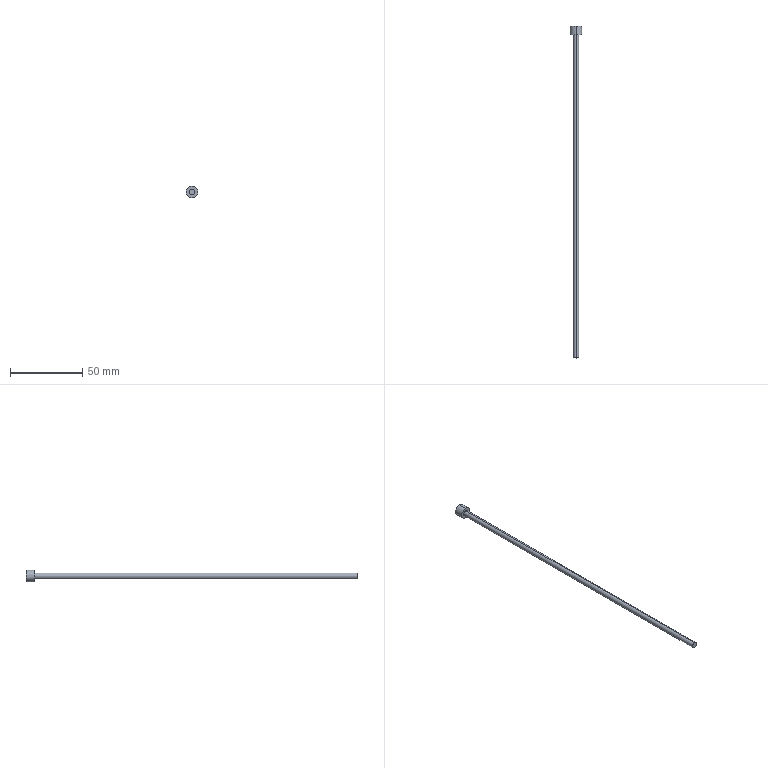Part | STEP file | 1 solid | 7 faces | box 8 x 229.999 x 8 mm | volume 3116 mm3 | cylinder 4 | plane 3 | commonest cylinder face diameters 4 x2 8 x2
STEP:
#1=CARTESIAN_POINT('',(0.,0.,0.));
#2=DIRECTION('',(0.,0.,1.));
#3=DIRECTION('',(1.,0.,0.));
#4=AXIS2_PLACEMENT_3D('',#1,#2,#3);
#5=CARTESIAN_POINT('',(-23.617,290.5,42.733));
#6=VERTEX_POINT('',#5);
#7=CARTESIAN_POINT('',(-23.617,290.5,50.733));
#8=VERTEX_POINT('',#7);
#9=CARTESIAN_POINT('',(-23.617,290.5,46.733));
#10=DIRECTION('',(0.,-1.,0.));
#11=DIRECTION('',(0.,0.,-1.));
#12=AXIS2_PLACEMENT_3D('',#9,#10,#11);
#13=CIRCLE('',#12,4.);
#14=CARTESIAN_POINT('',(-23.617,290.5,46.733));
#15=DIRECTION('',(0.,-1.,0.));
#16=DIRECTION('',(0.,0.,-1.));
#17=AXIS2_PLACEMENT_3D('',#14,#15,#16);
#18=CYLINDRICAL_SURFACE('',#17,4.);
#19=CARTESIAN_POINT('',(0.,0.));
#20=DIRECTION('',(1.,0.));
#21=VECTOR('',#20,1.);
#22=LINE('',#19,#21);
#23=(GEOMETRIC_REPRESENTATION_CONTEXT(2)PARAMETRIC_REPRESENTATION_CONTEXT()REPRESENTATION_CONTEXT('',''));
#24=DEFINITIONAL_REPRESENTATION('',(#22),#23);
#25=PCURVE('',#18,#24);
#26=CARTESIAN_POINT('',(-72.862,290.5,110.196));
#27=DIRECTION('',(0.,-1.,0.));
#28=DIRECTION('',(0.,0.,-1.));
#29=AXIS2_PLACEMENT_3D('',#26,#27,#28);
#30=PLANE('',#29);
#31=CARTESIAN_POINT('',(63.463,49.245));
#32=DIRECTION('',(1.,0.));
#33=AXIS2_PLACEMENT_2D('',#31,#32);
#34=CIRCLE('',#33,4.);
#35=(GEOMETRIC_REPRESENTATION_CONTEXT(2)PARAMETRIC_REPRESENTATION_CONTEXT()REPRESENTATION_CONTEXT('',''));
#36=DEFINITIONAL_REPRESENTATION('',(#34),#35);
#37=PCURVE('',#30,#36);
#38=SURFACE_CURVE('',#13,(#25,#37),.PCURVE_S1.);
#39=EDGE_CURVE('',#6,#8,#38,.T.);
#40=ORIENTED_EDGE('',*,*,#39,.T.);
#41=CARTESIAN_POINT('',(-23.617,284.5,50.733));
#42=VERTEX_POINT('',#41);
#43=CARTESIAN_POINT('',(-23.617,290.5,50.733));
#44=DIRECTION('',(0.,-1.,0.));
#45=VECTOR('',#44,1.);
#46=LINE('',#43,#45);
#47=CARTESIAN_POINT('',(3.142,0.));
#48=DIRECTION('',(0.,1.));
#49=VECTOR('',#48,1.);
#50=LINE('',#47,#49);
#51=(GEOMETRIC_REPRESENTATION_CONTEXT(2)PARAMETRIC_REPRESENTATION_CONTEXT()REPRESENTATION_CONTEXT('',''));
#52=DEFINITIONAL_REPRESENTATION('',(#50),#51);
#53=PCURVE('',#18,#52);
#54=CARTESIAN_POINT('',(-23.617,290.5,46.733));
#55=DIRECTION('',(0.,-1.,0.));
#56=DIRECTION('',(0.,0.,-1.));
#57=AXIS2_PLACEMENT_3D('',#54,#55,#56);
#58=CYLINDRICAL_SURFACE('',#57,4.);
#59=CARTESIAN_POINT('',(3.142,0.));
#60=DIRECTION('',(0.,1.));
#61=VECTOR('',#60,1.);
#62=LINE('',#59,#61);
#63=(GEOMETRIC_REPRESENTATION_CONTEXT(2)PARAMETRIC_REPRESENTATION_CONTEXT()REPRESENTATION_CONTEXT('',''));
#64=DEFINITIONAL_REPRESENTATION('',(#62),#63);
#65=PCURVE('',#58,#64);
#66=SURFACE_CURVE('',#46,(#53,#65),.PCURVE_S1.);
#67=EDGE_CURVE('',#8,#42,#66,.T.);
#68=ORIENTED_EDGE('',*,*,#67,.T.);
#69=CARTESIAN_POINT('',(-23.617,284.5,42.733));
#70=VERTEX_POINT('',#69);
#71=CARTESIAN_POINT('',(-23.617,284.5,46.733));
#72=DIRECTION('',(0.,1.,0.));
#73=DIRECTION('',(0.,0.,1.));
#74=AXIS2_PLACEMENT_3D('',#71,#72,#73);
#75=CIRCLE('',#74,4.);
#76=CARTESIAN_POINT('',(3.142,6.));
#77=DIRECTION('',(-1.,0.));
#78=VECTOR('',#77,1.);
#79=LINE('',#76,#78);
#80=(GEOMETRIC_REPRESENTATION_CONTEXT(2)PARAMETRIC_REPRESENTATION_CONTEXT()REPRESENTATION_CONTEXT('',''));
#81=DEFINITIONAL_REPRESENTATION('',(#79),#80);
#82=PCURVE('',#18,#81);
#83=CARTESIAN_POINT('',(-23.617,284.5,46.733));
#84=DIRECTION('',(0.,-1.,0.));
#85=DIRECTION('',(0.,0.,-1.));
#86=AXIS2_PLACEMENT_3D('',#83,#84,#85);
#87=PLANE('',#86);
#88=CARTESIAN_POINT('',(-4.,0.));
#89=CARTESIAN_POINT('',(-4.,6.928));
#90=CARTESIAN_POINT('',(2.,3.464));
#91=CARTESIAN_POINT('',(8.,0.));
#92=CARTESIAN_POINT('',(2.,-3.464));
#93=CARTESIAN_POINT('',(-4.,-6.928));
#94=CARTESIAN_POINT('',(-4.,0.));
#95=(BOUNDED_CURVE()B_SPLINE_CURVE(2,(#88,#89,#90,#91,#92,#93,#94),.UNSPECIFIED.,.T.,.F.)B_SPLINE_CURVE_WITH_KNOTS((1,2,2,2,2,1),(-2.094,0.,2.094,4.189,6.283,8.378),.UNSPECIFIED.)CURVE()GEOMETRIC_REPRESENTATION_ITEM()RATIONAL_B_SPLINE_CURVE((1.,0.5,1.,0.5,1.,0.5,1.))REPRESENTATION_ITEM(''));
#96=(GEOMETRIC_REPRESENTATION_CONTEXT(2)PARAMETRIC_REPRESENTATION_CONTEXT()REPRESENTATION_CONTEXT('',''));
#97=DEFINITIONAL_REPRESENTATION('',(#95),#96);
#98=PCURVE('',#87,#97);
#99=SURFACE_CURVE('',#75,(#82,#98),.PCURVE_S1.);
#100=EDGE_CURVE('',#42,#70,#99,.T.);
#101=ORIENTED_EDGE('',*,*,#100,.T.);
#102=CARTESIAN_POINT('',(-23.617,290.5,42.733));
#103=DIRECTION('',(0.,-1.,0.));
#104=VECTOR('',#103,1.);
#105=LINE('',#102,#104);
#106=CARTESIAN_POINT('',(0.,0.));
#107=DIRECTION('',(0.,1.));
#108=VECTOR('',#107,1.);
#109=LINE('',#106,#108);
#110=(GEOMETRIC_REPRESENTATION_CONTEXT(2)PARAMETRIC_REPRESENTATION_CONTEXT()REPRESENTATION_CONTEXT('',''));
#111=DEFINITIONAL_REPRESENTATION('',(#109),#110);
#112=PCURVE('',#18,#111);
#113=CARTESIAN_POINT('',(6.283,0.));
#114=DIRECTION('',(0.,1.));
#115=VECTOR('',#114,1.);
#116=LINE('',#113,#115);
#117=(GEOMETRIC_REPRESENTATION_CONTEXT(2)PARAMETRIC_REPRESENTATION_CONTEXT()REPRESENTATION_CONTEXT('',''));
#118=DEFINITIONAL_REPRESENTATION('',(#116),#117);
#119=PCURVE('',#58,#118);
#120=SURFACE_CURVE('',#105,(#112,#119),.PCURVE_S1.);
#121=EDGE_CURVE('',#6,#70,#120,.T.);
#122=ORIENTED_EDGE('',*,*,#121,.F.);
#123=EDGE_LOOP('',(#40,#68,#101,#122));
#124=FACE_BOUND('',#123,.T.);
#125=ADVANCED_FACE('',(#124),#18,.T.);
#126=CARTESIAN_POINT('',(-23.617,284.5,48.733));
#127=VERTEX_POINT('',#126);
#128=CARTESIAN_POINT('',(-23.617,284.5,44.733));
#129=VERTEX_POINT('',#128);
#130=CARTESIAN_POINT('',(-23.617,284.5,46.733));
#131=DIRECTION('',(0.,1.,0.));
#132=DIRECTION('',(0.,0.,-1.));
#133=AXIS2_PLACEMENT_3D('',#130,#131,#132);
#134=CIRCLE('',#133,2.);
#135=CARTESIAN_POINT('',(-23.617,220.5,46.733));
#136=DIRECTION('',(0.,-1.,0.));
#137=DIRECTION('',(0.,0.,-1.));
#138=AXIS2_PLACEMENT_3D('',#135,#136,#137);
#139=CYLINDRICAL_SURFACE('',#138,2.);
#140=CARTESIAN_POINT('',(6.283,-64.));
#141=DIRECTION('',(-1.,0.));
#142=VECTOR('',#141,1.);
#143=LINE('',#140,#142);
#144=(GEOMETRIC_REPRESENTATION_CONTEXT(2)PARAMETRIC_REPRESENTATION_CONTEXT()REPRESENTATION_CONTEXT('',''));
#145=DEFINITIONAL_REPRESENTATION('',(#143),#144);
#146=PCURVE('',#139,#145);
#147=CARTESIAN_POINT('',(2.,0.));
#148=CARTESIAN_POINT('',(2.,-3.464));
#149=CARTESIAN_POINT('',(-1.,-1.732));
#150=CARTESIAN_POINT('',(-4.,0.));
#151=CARTESIAN_POINT('',(-1.,1.732));
#152=CARTESIAN_POINT('',(2.,3.464));
#153=CARTESIAN_POINT('',(2.,0.));
#154=(BOUNDED_CURVE()B_SPLINE_CURVE(2,(#147,#148,#149,#150,#151,#152,#153),.UNSPECIFIED.,.T.,.F.)B_SPLINE_CURVE_WITH_KNOTS((1,2,2,2,2,1),(-2.094,0.,2.094,4.189,6.283,8.378),.UNSPECIFIED.)CURVE()GEOMETRIC_REPRESENTATION_ITEM()RATIONAL_B_SPLINE_CURVE((1.,0.5,1.,0.5,1.,0.5,1.))REPRESENTATION_ITEM(''));
#155=(GEOMETRIC_REPRESENTATION_CONTEXT(2)PARAMETRIC_REPRESENTATION_CONTEXT()REPRESENTATION_CONTEXT('',''));
#156=DEFINITIONAL_REPRESENTATION('',(#154),#155);
#157=PCURVE('',#87,#156);
#158=SURFACE_CURVE('',#134,(#146,#157),.PCURVE_S1.);
#159=EDGE_CURVE('',#127,#129,#158,.T.);
#160=ORIENTED_EDGE('',*,*,#159,.F.);
#161=CARTESIAN_POINT('',(-23.617,60.501,48.733));
#162=VERTEX_POINT('',#161);
#163=CARTESIAN_POINT('',(-23.617,220.5,48.733));
#164=DIRECTION('',(0.,-1.,0.));
#165=VECTOR('',#164,1.);
#166=LINE('',#163,#165);
#167=CARTESIAN_POINT('',(3.142,0.));
#168=DIRECTION('',(0.,1.));
#169=VECTOR('',#168,1.);
#170=LINE('',#167,#169);
#171=(GEOMETRIC_REPRESENTATION_CONTEXT(2)PARAMETRIC_REPRESENTATION_CONTEXT()REPRESENTATION_CONTEXT('',''));
#172=DEFINITIONAL_REPRESENTATION('',(#170),#171);
#173=PCURVE('',#139,#172);
#174=CARTESIAN_POINT('',(-23.617,220.5,46.733));
#175=DIRECTION('',(0.,-1.,0.));
#176=DIRECTION('',(0.,0.,-1.));
#177=AXIS2_PLACEMENT_3D('',#174,#175,#176);
#178=CYLINDRICAL_SURFACE('',#177,2.);
#179=CARTESIAN_POINT('',(3.142,0.));
#180=DIRECTION('',(0.,1.));
#181=VECTOR('',#180,1.);
#182=LINE('',#179,#181);
#183=(GEOMETRIC_REPRESENTATION_CONTEXT(2)PARAMETRIC_REPRESENTATION_CONTEXT()REPRESENTATION_CONTEXT('',''));
#184=DEFINITIONAL_REPRESENTATION('',(#182),#183);
#185=PCURVE('',#178,#184);
#186=SURFACE_CURVE('',#166,(#173,#185),.PCURVE_S1.);
#187=EDGE_CURVE('',#127,#162,#186,.T.);
#188=ORIENTED_EDGE('',*,*,#187,.T.);
#189=CARTESIAN_POINT('',(-23.617,60.501,44.733));
#190=VERTEX_POINT('',#189);
#191=CARTESIAN_POINT('',(-23.617,60.501,46.733));
#192=DIRECTION('',(0.,-1.,0.));
#193=DIRECTION('',(0.,0.,1.));
#194=AXIS2_PLACEMENT_3D('',#191,#192,#193);
#195=CIRCLE('',#194,2.);
#196=CARTESIAN_POINT('',(-3.142,159.999));
#197=DIRECTION('',(1.,0.));
#198=VECTOR('',#197,1.);
#199=LINE('',#196,#198);
#200=(GEOMETRIC_REPRESENTATION_CONTEXT(2)PARAMETRIC_REPRESENTATION_CONTEXT()REPRESENTATION_CONTEXT('',''));
#201=DEFINITIONAL_REPRESENTATION('',(#199),#200);
#202=PCURVE('',#139,#201);
#203=CARTESIAN_POINT('',(-23.617,60.501,46.733));
#204=DIRECTION('',(0.,1.,0.));
#205=DIRECTION('',(0.,0.,1.));
#206=AXIS2_PLACEMENT_3D('',#203,#204,#205);
#207=PLANE('',#206);
#208=CARTESIAN_POINT('',(2.,0.));
#209=CARTESIAN_POINT('',(2.,-3.464));
#210=CARTESIAN_POINT('',(-1.,-1.732));
#211=CARTESIAN_POINT('',(-4.,0.));
#212=CARTESIAN_POINT('',(-1.,1.732));
#213=CARTESIAN_POINT('',(2.,3.464));
#214=CARTESIAN_POINT('',(2.,0.));
#215=(BOUNDED_CURVE()B_SPLINE_CURVE(2,(#208,#209,#210,#211,#212,#213,#214),.UNSPECIFIED.,.T.,.F.)B_SPLINE_CURVE_WITH_KNOTS((1,2,2,2,2,1),(-2.094,0.,2.094,4.189,6.283,8.378),.UNSPECIFIED.)CURVE()GEOMETRIC_REPRESENTATION_ITEM()RATIONAL_B_SPLINE_CURVE((1.,0.5,1.,0.5,1.,0.5,1.))REPRESENTATION_ITEM(''));
#216=(GEOMETRIC_REPRESENTATION_CONTEXT(2)PARAMETRIC_REPRESENTATION_CONTEXT()REPRESENTATION_CONTEXT('',''));
#217=DEFINITIONAL_REPRESENTATION('',(#215),#216);
#218=PCURVE('',#207,#217);
#219=SURFACE_CURVE('',#195,(#202,#218),.PCURVE_S1.);
#220=EDGE_CURVE('',#190,#162,#219,.T.);
#221=ORIENTED_EDGE('',*,*,#220,.F.);
#222=CARTESIAN_POINT('',(-23.617,220.5,44.733));
#223=DIRECTION('',(0.,-1.,0.));
#224=VECTOR('',#223,1.);
#225=LINE('',#222,#224);
#226=CARTESIAN_POINT('',(0.,0.));
#227=DIRECTION('',(0.,1.));
#228=VECTOR('',#227,1.);
#229=LINE('',#226,#228);
#230=(GEOMETRIC_REPRESENTATION_CONTEXT(2)PARAMETRIC_REPRESENTATION_CONTEXT()REPRESENTATION_CONTEXT('',''));
#231=DEFINITIONAL_REPRESENTATION('',(#229),#230);
#232=PCURVE('',#139,#231);
#233=CARTESIAN_POINT('',(6.283,0.));
#234=DIRECTION('',(0.,1.));
#235=VECTOR('',#234,1.);
#236=LINE('',#233,#235);
#237=(GEOMETRIC_REPRESENTATION_CONTEXT(2)PARAMETRIC_REPRESENTATION_CONTEXT()REPRESENTATION_CONTEXT('',''));
#238=DEFINITIONAL_REPRESENTATION('',(#236),#237);
#239=PCURVE('',#178,#238);
#240=SURFACE_CURVE('',#225,(#232,#239),.PCURVE_S1.);
#241=EDGE_CURVE('',#129,#190,#240,.T.);
#242=ORIENTED_EDGE('',*,*,#241,.F.);
#243=EDGE_LOOP('',(#160,#188,#221,#242));
#244=FACE_BOUND('',#243,.T.);
#245=ADVANCED_FACE('',(#244),#139,.T.);
#246=ORIENTED_EDGE('',*,*,#220,.T.);
#247=CARTESIAN_POINT('',(-23.617,60.501,46.733));
#248=DIRECTION('',(0.,-1.,0.));
#249=DIRECTION('',(0.,0.,1.));
#250=AXIS2_PLACEMENT_3D('',#247,#248,#249);
#251=CIRCLE('',#250,2.);
#252=CARTESIAN_POINT('',(2.,0.));
#253=CARTESIAN_POINT('',(2.,-3.464));
#254=CARTESIAN_POINT('',(-1.,-1.732));
#255=CARTESIAN_POINT('',(-4.,0.));
#256=CARTESIAN_POINT('',(-1.,1.732));
#257=CARTESIAN_POINT('',(2.,3.464));
#258=CARTESIAN_POINT('',(2.,0.));
#259=(BOUNDED_CURVE()B_SPLINE_CURVE(2,(#252,#253,#254,#255,#256,#257,#258),.UNSPECIFIED.,.T.,.F.)B_SPLINE_CURVE_WITH_KNOTS((1,2,2,2,2,1),(-2.094,0.,2.094,4.189,6.283,8.378),.UNSPECIFIED.)CURVE()GEOMETRIC_REPRESENTATION_ITEM()RATIONAL_B_SPLINE_CURVE((1.,0.5,1.,0.5,1.,0.5,1.))REPRESENTATION_ITEM(''));
#260=(GEOMETRIC_REPRESENTATION_CONTEXT(2)PARAMETRIC_REPRESENTATION_CONTEXT()REPRESENTATION_CONTEXT('',''));
#261=DEFINITIONAL_REPRESENTATION('',(#259),#260);
#262=PCURVE('',#207,#261);
#263=CARTESIAN_POINT('',(3.142,159.999));
#264=DIRECTION('',(1.,0.));
#265=VECTOR('',#264,1.);
#266=LINE('',#263,#265);
#267=(GEOMETRIC_REPRESENTATION_CONTEXT(2)PARAMETRIC_REPRESENTATION_CONTEXT()REPRESENTATION_CONTEXT('',''));
#268=DEFINITIONAL_REPRESENTATION('',(#266),#267);
#269=PCURVE('',#178,#268);
#270=SURFACE_CURVE('',#251,(#262,#269),.PCURVE_S1.);
#271=EDGE_CURVE('',#162,#190,#270,.T.);
#272=ORIENTED_EDGE('',*,*,#271,.T.);
#273=EDGE_LOOP('',(#246,#272));
#274=FACE_BOUND('',#273,.T.);
#275=ADVANCED_FACE('',(#274),#207,.F.);
#276=ORIENTED_EDGE('',*,*,#187,.F.);
#277=CARTESIAN_POINT('',(-23.617,284.5,46.733));
#278=DIRECTION('',(0.,1.,0.));
#279=DIRECTION('',(0.,0.,-1.));
#280=AXIS2_PLACEMENT_3D('',#277,#278,#279);
#281=CIRCLE('',#280,2.);
#282=CARTESIAN_POINT('',(6.283,-64.));
#283=DIRECTION('',(-1.,0.));
#284=VECTOR('',#283,1.);
#285=LINE('',#282,#284);
#286=(GEOMETRIC_REPRESENTATION_CONTEXT(2)PARAMETRIC_REPRESENTATION_CONTEXT()REPRESENTATION_CONTEXT('',''));
#287=DEFINITIONAL_REPRESENTATION('',(#285),#286);
#288=PCURVE('',#178,#287);
#289=CARTESIAN_POINT('',(2.,0.));
#290=CARTESIAN_POINT('',(2.,-3.464));
#291=CARTESIAN_POINT('',(-1.,-1.732));
#292=CARTESIAN_POINT('',(-4.,0.));
#293=CARTESIAN_POINT('',(-1.,1.732));
#294=CARTESIAN_POINT('',(2.,3.464));
#295=CARTESIAN_POINT('',(2.,0.));
#296=(BOUNDED_CURVE()B_SPLINE_CURVE(2,(#289,#290,#291,#292,#293,#294,#295),.UNSPECIFIED.,.T.,.F.)B_SPLINE_CURVE_WITH_KNOTS((1,2,2,2,2,1),(-2.094,0.,2.094,4.189,6.283,8.378),.UNSPECIFIED.)CURVE()GEOMETRIC_REPRESENTATION_ITEM()RATIONAL_B_SPLINE_CURVE((1.,0.5,1.,0.5,1.,0.5,1.))REPRESENTATION_ITEM(''));
#297=(GEOMETRIC_REPRESENTATION_CONTEXT(2)PARAMETRIC_REPRESENTATION_CONTEXT()REPRESENTATION_CONTEXT('',''));
#298=DEFINITIONAL_REPRESENTATION('',(#296),#297);
#299=PCURVE('',#87,#298);
#300=SURFACE_CURVE('',#281,(#288,#299),.PCURVE_S1.);
#301=EDGE_CURVE('',#129,#127,#300,.T.);
#302=ORIENTED_EDGE('',*,*,#301,.F.);
#303=ORIENTED_EDGE('',*,*,#241,.T.);
#304=ORIENTED_EDGE('',*,*,#271,.F.);
#305=EDGE_LOOP('',(#276,#302,#303,#304));
#306=FACE_BOUND('',#305,.T.);
#307=ADVANCED_FACE('',(#306),#178,.T.);
#308=ORIENTED_EDGE('',*,*,#301,.T.);
#309=ORIENTED_EDGE('',*,*,#159,.T.);
#310=EDGE_LOOP('',(#308,#309));
#311=FACE_BOUND('',#310,.T.);
#312=CARTESIAN_POINT('',(-23.617,284.5,46.733));
#313=DIRECTION('',(0.,1.,0.));
#314=DIRECTION('',(0.,0.,1.));
#315=AXIS2_PLACEMENT_3D('',#312,#313,#314);
#316=CIRCLE('',#315,4.);
#317=CARTESIAN_POINT('',(-4.,0.));
#318=CARTESIAN_POINT('',(-4.,6.928));
#319=CARTESIAN_POINT('',(2.,3.464));
#320=CARTESIAN_POINT('',(8.,0.));
#321=CARTESIAN_POINT('',(2.,-3.464));
#322=CARTESIAN_POINT('',(-4.,-6.928));
#323=CARTESIAN_POINT('',(-4.,0.));
#324=(BOUNDED_CURVE()B_SPLINE_CURVE(2,(#317,#318,#319,#320,#321,#322,#323),.UNSPECIFIED.,.T.,.F.)B_SPLINE_CURVE_WITH_KNOTS((1,2,2,2,2,1),(-2.094,0.,2.094,4.189,6.283,8.378),.UNSPECIFIED.)CURVE()GEOMETRIC_REPRESENTATION_ITEM()RATIONAL_B_SPLINE_CURVE((1.,0.5,1.,0.5,1.,0.5,1.))REPRESENTATION_ITEM(''));
#325=(GEOMETRIC_REPRESENTATION_CONTEXT(2)PARAMETRIC_REPRESENTATION_CONTEXT()REPRESENTATION_CONTEXT('',''));
#326=DEFINITIONAL_REPRESENTATION('',(#324),#325);
#327=PCURVE('',#87,#326);
#328=CARTESIAN_POINT('',(9.425,6.));
#329=DIRECTION('',(-1.,0.));
#330=VECTOR('',#329,1.);
#331=LINE('',#328,#330);
#332=(GEOMETRIC_REPRESENTATION_CONTEXT(2)PARAMETRIC_REPRESENTATION_CONTEXT()REPRESENTATION_CONTEXT('',''));
#333=DEFINITIONAL_REPRESENTATION('',(#331),#332);
#334=PCURVE('',#58,#333);
#335=SURFACE_CURVE('',#316,(#327,#334),.PCURVE_S1.);
#336=EDGE_CURVE('',#70,#42,#335,.T.);
#337=ORIENTED_EDGE('',*,*,#336,.F.);
#338=ORIENTED_EDGE('',*,*,#100,.F.);
#339=EDGE_LOOP('',(#337,#338));
#340=FACE_BOUND('',#339,.T.);
#341=ADVANCED_FACE('',(#311,#340),#87,.T.);
#342=ORIENTED_EDGE('',*,*,#67,.F.);
#343=CARTESIAN_POINT('',(-23.617,290.5,46.733));
#344=DIRECTION('',(0.,-1.,0.));
#345=DIRECTION('',(0.,0.,-1.));
#346=AXIS2_PLACEMENT_3D('',#343,#344,#345);
#347=CIRCLE('',#346,4.);
#348=CARTESIAN_POINT('',(0.,0.));
#349=DIRECTION('',(1.,0.));
#350=VECTOR('',#349,1.);
#351=LINE('',#348,#350);
#352=(GEOMETRIC_REPRESENTATION_CONTEXT(2)PARAMETRIC_REPRESENTATION_CONTEXT()REPRESENTATION_CONTEXT('',''));
#353=DEFINITIONAL_REPRESENTATION('',(#351),#352);
#354=PCURVE('',#58,#353);
#355=CARTESIAN_POINT('',(63.463,49.245));
#356=DIRECTION('',(1.,0.));
#357=AXIS2_PLACEMENT_2D('',#355,#356);
#358=CIRCLE('',#357,4.);
#359=(GEOMETRIC_REPRESENTATION_CONTEXT(2)PARAMETRIC_REPRESENTATION_CONTEXT()REPRESENTATION_CONTEXT('',''));
#360=DEFINITIONAL_REPRESENTATION('',(#358),#359);
#361=PCURVE('',#30,#360);
#362=SURFACE_CURVE('',#347,(#354,#361),.PCURVE_S1.);
#363=EDGE_CURVE('',#8,#6,#362,.T.);
#364=ORIENTED_EDGE('',*,*,#363,.T.);
#365=ORIENTED_EDGE('',*,*,#121,.T.);
#366=ORIENTED_EDGE('',*,*,#336,.T.);
#367=EDGE_LOOP('',(#342,#364,#365,#366));
#368=FACE_BOUND('',#367,.T.);
#369=ADVANCED_FACE('',(#368),#58,.T.);
#370=ORIENTED_EDGE('',*,*,#39,.F.);
#371=ORIENTED_EDGE('',*,*,#363,.F.);
#372=EDGE_LOOP('',(#370,#371));
#373=FACE_BOUND('',#372,.T.);
#374=ADVANCED_FACE('',(#373),#30,.F.);
#375=CLOSED_SHELL('',(#125,#245,#275,#307,#341,#369,#374));
#376=MANIFOLD_SOLID_BREP('',#375);
#377=(LENGTH_UNIT()NAMED_UNIT(*)SI_UNIT(.MILLI.,.METRE.));
#378=UNCERTAINTY_MEASURE_WITH_UNIT(LENGTH_MEASURE(0.0000001),#377,'','');
#379=(NAMED_UNIT(*)PLANE_ANGLE_UNIT()SI_UNIT($,.RADIAN.));
#380=(NAMED_UNIT(*)SI_UNIT($,.STERADIAN.)SOLID_ANGLE_UNIT());
#381=(GEOMETRIC_REPRESENTATION_CONTEXT(3)GLOBAL_UNCERTAINTY_ASSIGNED_CONTEXT((#378))GLOBAL_UNIT_ASSIGNED_CONTEXT((#377,#379,#380))REPRESENTATION_CONTEXT('',''));
#382=ADVANCED_BREP_SHAPE_REPRESENTATION('',(#4,#376),#381);